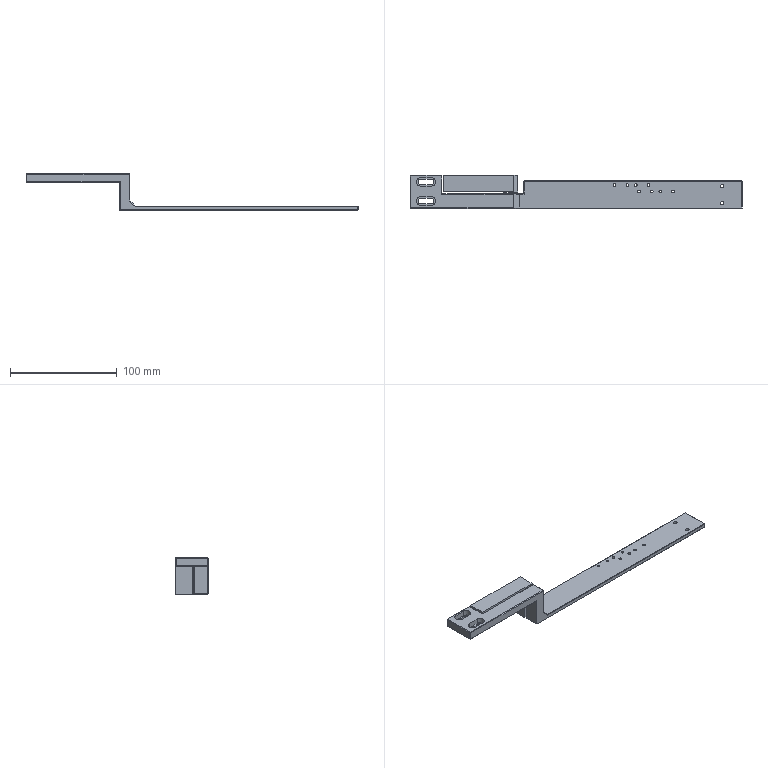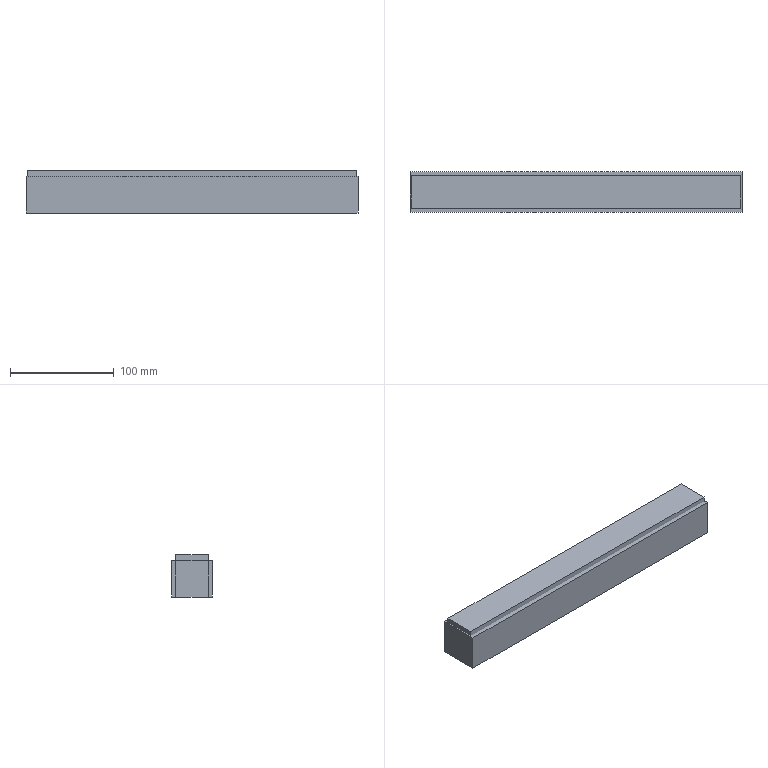CAM job | NX | 3+2 milling, drilling | part box 311.5 x 31 x 34.5 mm | stock box 319.5 x 39 x 40.5 mm
Tools:
number,name,description,diameter,corner_radius,flute_length,length,flutes
1,D63,Milling Tool-5 Parameters,63.0,0.0,50.0,75.0,2
2,D10,Milling Tool-5 Parameters,10.0,0.0,50.0,75.0,2
4,D6,Milling Tool-5 Parameters,6.0,0.0,50.0,75.0,2
6,D4,Milling Tool-5 Parameters,4.0,0.0,50.0,75.0,2
9,D6A45,Milling Tool-5 Parameters,6.0,0.0,3.0,3.0,2
12,3.2ZT,Drilling Tool,3.2,0.0,35.0,50.0,2
10,2.5ZT,Drilling Tool,2.4,0.0,35.0,50.0,2
20,R0.75,Milling Tool-5 Parameters,1.5,0.75,50.0,75.0,2
Operations:
program,operation,operation_type,tool,method,geometry_group,spindle_rpm,surface_speed,feed_per_tooth,feed_cut,feed_plunge,cut_length_mm,path_length_mm,cut_time_min,machine_time_min
1-315-40-35毛胚-虎钳,FLOOR_WALL,VolumeBased25DMillingOperation,D63,METHOD,A,6500.0,0.0,0.0,1250.0,100.0,394.5,448.5,0.3156,0.321
1-315-40-35毛胚-虎钳,ADAPTIVE_MILLING,CavityMilling,D10,METHOD,A,7000.0,219.0,0.1429,2000.0,1000.0,10750.126,17068.391,5.405,6.037
1-315-40-35毛胚-虎钳,FLOOR_WALL_1,VolumeBased25DMillingOperation,D10,METHOD,A,7000.0,219.0,0.1786,2500.0,1000.0,19768.836,20173.88,7.915,7.955
1-315-40-35毛胚-虎钳,FLOOR_WALL_1_COPY,VolumeBased25DMillingOperation,D10,METHOD,A,7000.0,219.0,0.1786,2500.0,1000.0,9687.871,9802.671,3.879,3.89
1-315-40-35毛胚-虎钳,ZLEVEL_PROFILE_COPY_COPY_1_COPY,ZLevelMilling,D10,METHOD,A,6500.0,326.0,0.0769,1000.0,1000.0,593.144,701.368,0.5931,0.604
1-315-40-35毛胚-虎钳,ZLEVEL_PROFILE_COPY_COPY_1,ZLevelMilling,D10,METHOD,A,6500.0,326.0,0.0769,1000.0,1000.0,722.227,848.227,0.7222,0.7348
1-315-40-35毛胚-虎钳,FLOOR_WALL_1_COPY_COPY,VolumeBased25DMillingOperation,D10,METHOD,A,7000.0,219.0,0.0714,1000.0,1000.0,1681.221,2189.004,1.681,1.747
1-315-40-35毛胚-虎钳,ZLEVEL_PROFILE_1,ZLevelMilling,D10,METHOD,A,7000.0,131.0,0.1786,2500.0,1000.0,3795.161,3908.218,1.52,1.532
1-315-40-35毛胚-虎钳,ZLEVEL_PROFILE,ZLevelMilling,D6,METHOD,A,7000.0,131.0,0.1429,2000.0,1000.0,630.343,772.602,0.3534,0.3676
1-315-40-35毛胚-虎钳,ZLEVEL_PROFILE_COPY_COPY_1_COPY_1,ZLevelMilling,D6,METHOD,A,6500.0,326.0,0.0769,1000.0,1000.0,63.509,218.342,0.0635,0.079
1-315-40-35毛胚-虎钳,ZLEVEL_PROFILE_COPY,ZLevelMilling,D4,METHOD,A,7000.0,87.0,0.1,1400.0,1000.0,479.207,637.276,0.3628,0.3786
1-315-40-35毛胚-虎钳,DRILLING,Operation,D6A45,METHOD,A,4000.0,75.0,0.0312,250.0,0.0,40.0,358.409,0.16,0.1918
1-315-40-35毛胚-虎钳,DRILLING_COPY_1,Operation,3.2ZT,METHOD,A,2000.0,20.0,0.05,200.0,0.0,18.923,178.124,0.0946,0.1105
1-315-40-35毛胚-虎钳,DRILLING_COPY_1_COPY,Operation,2.5ZT,METHOD,A,2000.0,15.0,0.0375,150.0,0.0,73.768,357.101,0.4918,0.5201
1-315-40-35毛胚-虎钳,ZLEVEL_PROFILE_COPY_1_COPY_COPY_COPY_COPY,ZLevelMilling,D6A45,METHOD,A,7000.0,131.0,0.0714,1000.0,1000.0,520.164,949.518,0.5202,0.5631
1-315-40-35毛胚-虎钳,ZLEVEL_PROFILE_COPY_1_COPY_COPY_COPY_COPY_COPY,ZLevelMilling,D6A45,METHOD,A,7000.0,131.0,0.0714,1000.0,1000.0,495.67,2352.21,0.4957,0.6813
1-315-40-35毛胚-虎钳,PLANAR_TEXT,Engraving,R0.75,METHOD,A,7000.0,0.0,0.0,1000.0,500.0,668.491,4706.242,0.7444,1.148
2-315-40-35毛胚-虎钳,FLOOR_WALL_COPY,VolumeBased25DMillingOperation,D63,METHOD,B,6500.0,0.0,0.0,1250.0,100.0,2355.0,4581.502,1.884,2.107
2-315-40-35毛胚-虎钳,FLOOR_WALL_1_COPY_1,VolumeBased25DMillingOperation,D10,METHOD,B,7000.0,219.0,0.1786,2500.0,1000.0,9328.4,9603.3,3.739,3.766
2-315-40-35毛胚-虎钳,ZLEVEL_PROFILE_COPY_COPY_1_COPY_COPY,ZLevelMilling,D10,METHOD,B,6500.0,326.0,0.0769,1000.0,1000.0,100.406,244.5,0.1004,0.1148
2-315-40-35毛胚-虎钳,FLOOR_WALL_1_COPY_COPY_COPY_1,VolumeBased25DMillingOperation,D10,METHOD,B,7000.0,219.0,0.0714,1000.0,1000.0,912.657,1071.158,0.9127,0.9314
2-315-40-35毛胚-虎钳,ZLEVEL_PROFILE_COPY_1_COPY_COPY_COPY_COPY_COPY_1,ZLevelMilling,D6A45,METHOD,B,7000.0,131.0,0.0714,1000.0,1000.0,607.614,1885.542,0.6076,0.7354
2-315-40-35毛胚-虎钳,ZLEVEL_PROFILE_COPY_1_COPY_COPY_COPY_COPY_COPY_1_COPY,ZLevelMilling,D6A45,METHOD,B,7000.0,131.0,0.0714,1000.0,1000.0,414.264,1003.628,0.4143,0.4732
3,FLOOR_WALL_1_COPY_2,VolumeBased25DMillingOperation,D10,METHOD,C,7000.0,219.0,0.1786,2500.0,1000.0,7293.945,8516.145,2.979,3.101
3,FLOOR_WALL_1_COPY_COPY_COPY,VolumeBased25DMillingOperation,D10,METHOD,C,7000.0,219.0,0.0714,1000.0,1000.0,489.501,827.784,0.4895,0.5297
3,ZLEVEL_PROFILE_COPY_1_COPY_COPY_COPY_COPY_COPY_1_COPY_1,ZLevelMilling,D6A45,METHOD,C,7000.0,131.0,0.0714,1000.0,1000.0,201.095,401.115,0.2011,0.2211